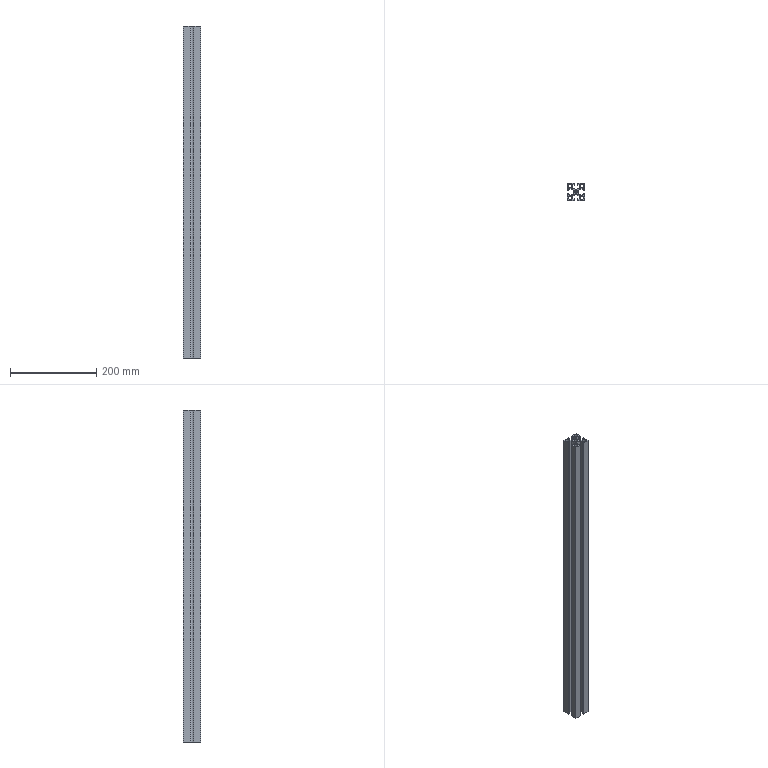Part | STEP file | Frame aluminum channel 2 | 1 solid | 49 faces | box 40 x 40 x 770 mm | volume 498412 mm3 | plane 34 | cylinder 15 | commonest cylinder face diameters 9 x8 19.803 x5 7 x2